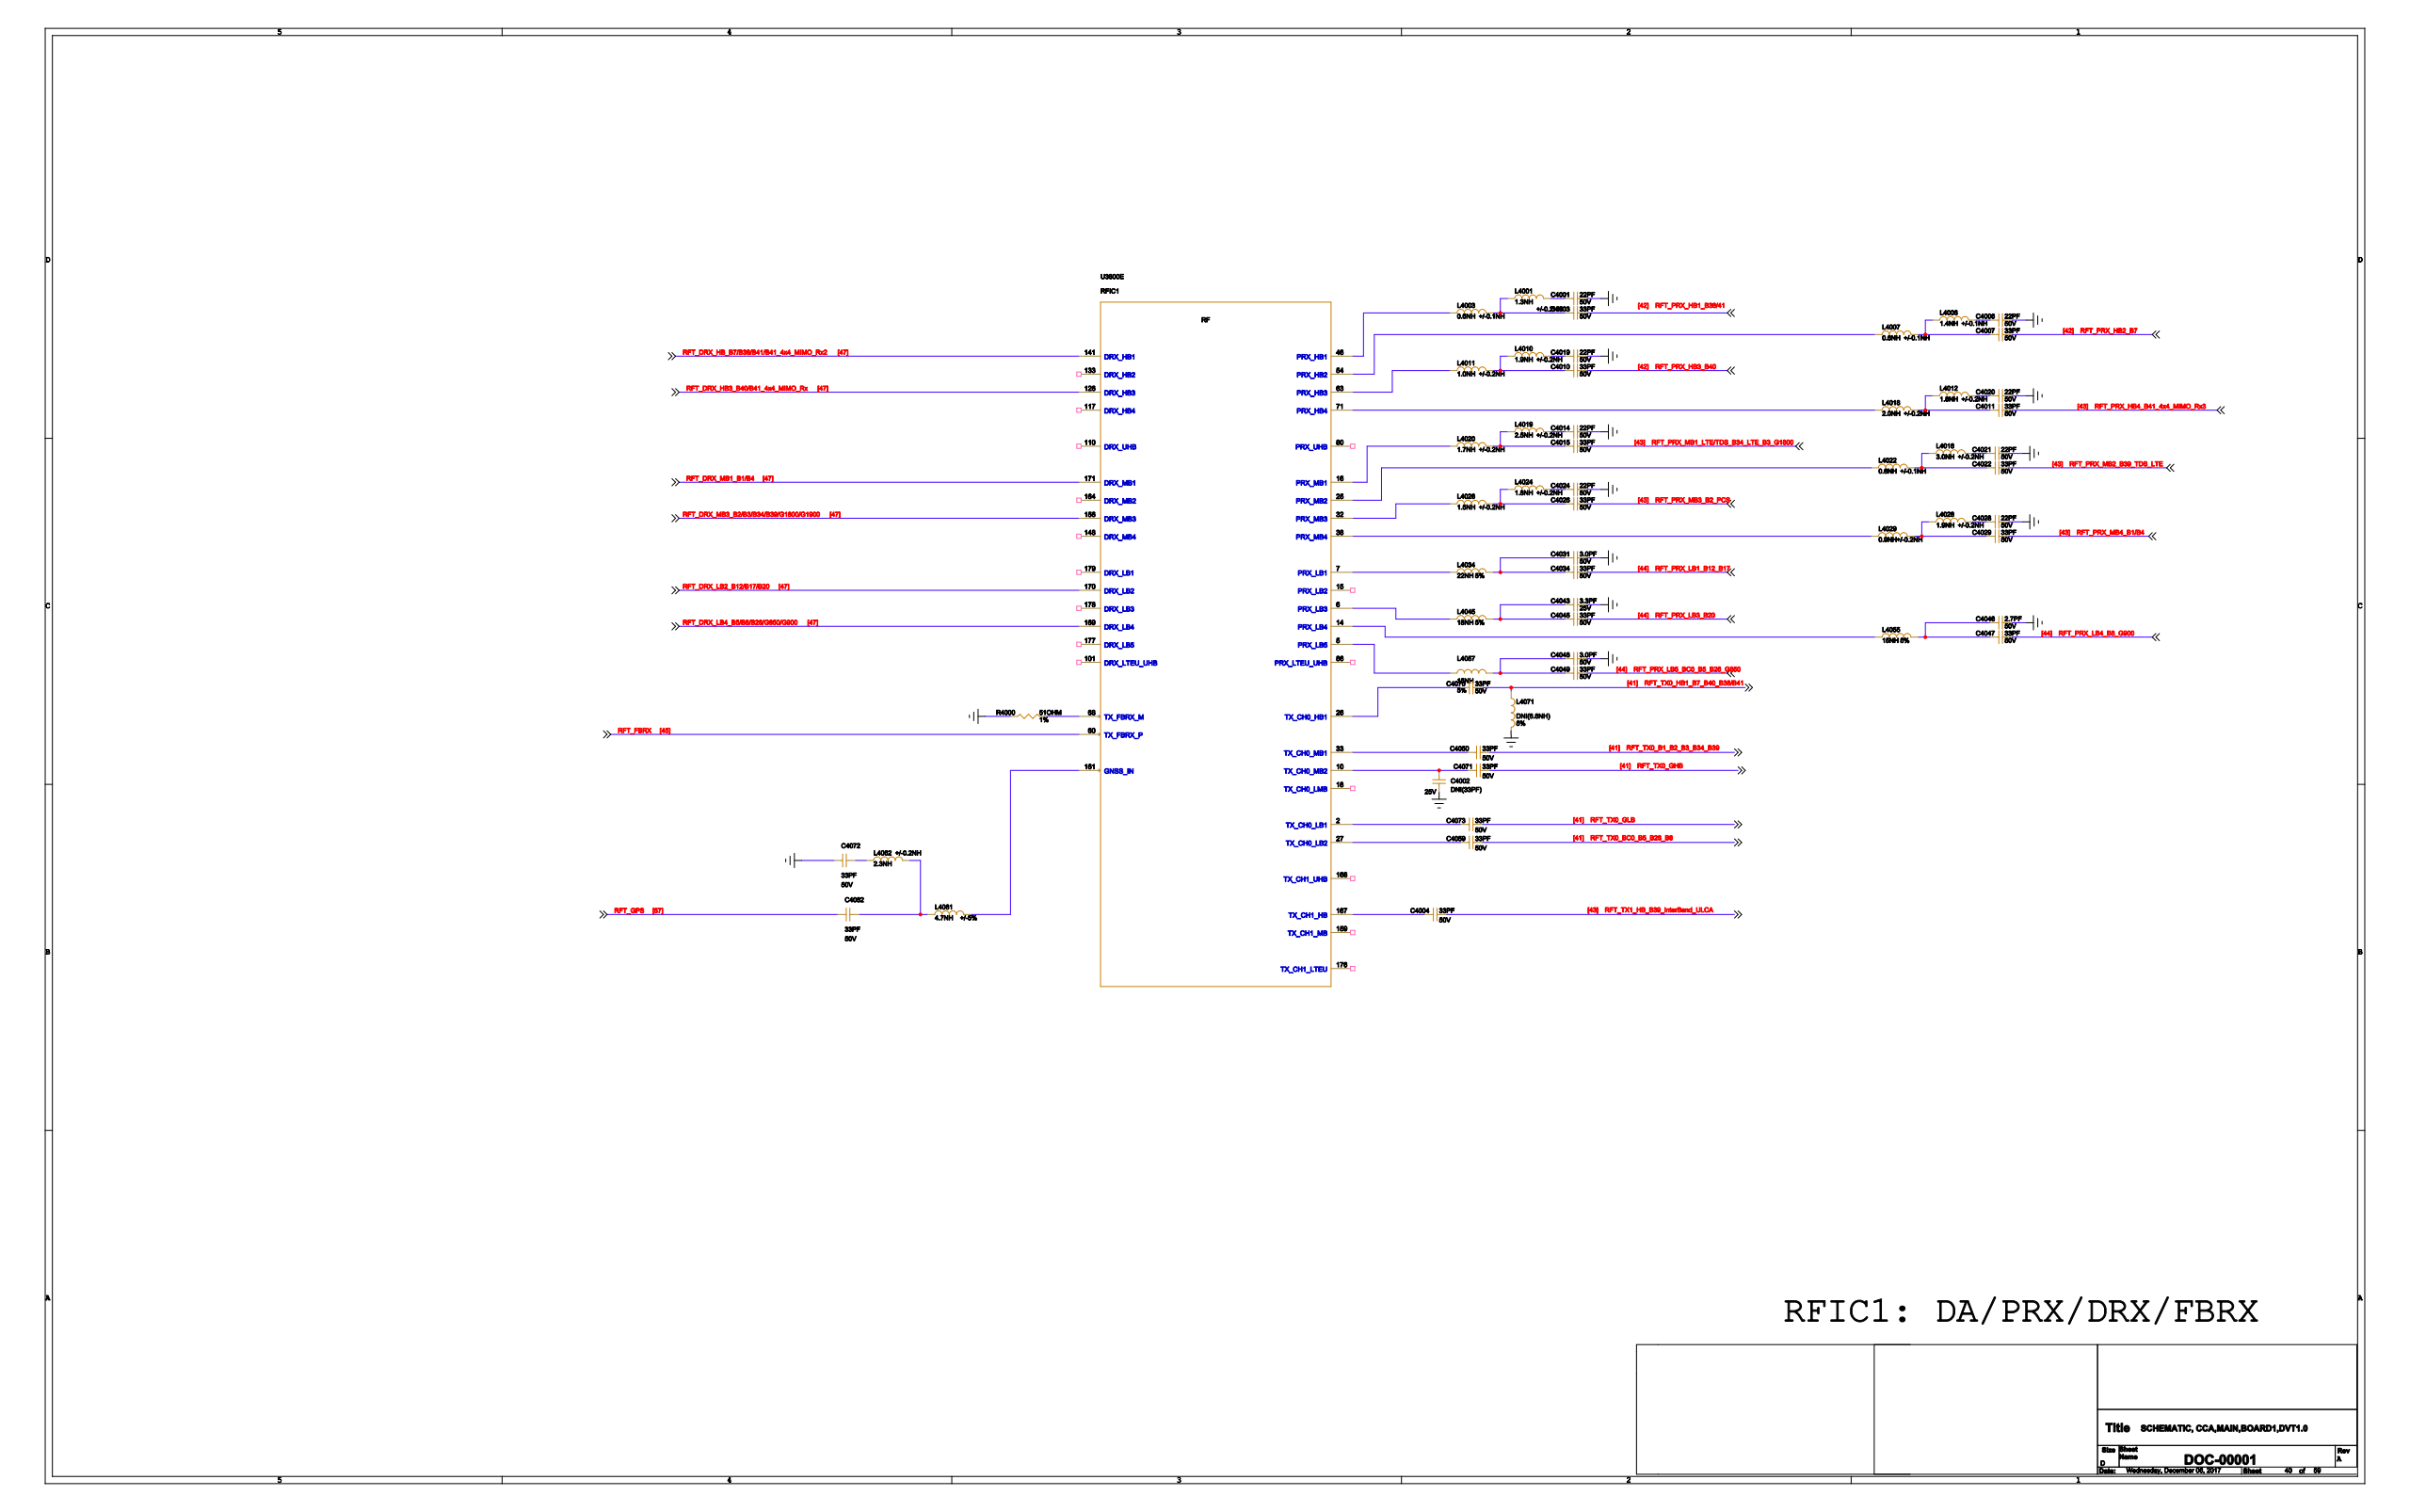Circuit board | KiCad | 1657 parts | 1365 nets | one sheet of the schematic
Parts on this sheet (reference | value | footprint):
C4001
C4002
C4003
C4004
C4006
C4007
C4010
C4011
C4014
C4015
C4019
C4020
C4021
C4022
C4024
C4026
C4028
C4029
C4031
C4034
C4043
C4045
C4046
C4047
C4048
C4049
C4050
C4059
C4062
C4070
C4071
C4072
C4073
L4001
L4003
L4006
L4007
L4010
L4011
L4012
L4016
L4018
L4019
L4020
L4022
L4024
L4026
L4028
L4029
L4034
L4045
L4055
L4057
L4061
L4062
L4071
R4000
U3800
Nets of these parts (net: part-pin ...):
GND: C4001-2 C4002-1 C4006-2 C4014-2 C4019-2 C4020-2 C4021-2 C4024-2 C4028-2 C4031-2 C4043-2 C4046-2 C4048-2 C4072-1 L4071-2 R4000-1 U3800-1 U3800-4 U3800-40
N42474209: C4031-1 C4034-1 L4034-2
RX_LB1_B12_B17: C4034-2
N42473365: C4073-1 U3800-2
RFT_TX0_GLB: C4073-2
N42473857: L4022-1 U3800-25
N42474033: C4022-1 L4016-1 L4022-2
N42474137: C4024-1 L4024-2
N42473873: L4029-1 U3800-38
N42474149: C4029-1 L4028-1 L4029-2
N42474119: C4026-1 L4024-1 L4026-2
N42473849: C4019-1 L4010-2
N42473276: C4002-2 C4071-1 U3800-10
RFT_TX0_GHB: C4071-2
N42473340: C4070-1 U3800-26
B7_B40_B38/B41: C4070-2 L4071-1
N42473847: C4010-1 L4010-1 L4011-2
FT_PRX_HB3_B40: C4010-2
RX_LB4_B8_G900: C4047-2
N42474251: C4043-1 C4045-1 L4045-2
N42473389: C4050-1 U3800-33
_B2_B3_B34_B39: C4050-2
PRX_MB3_B2_PCS: C4026-2
RFT_FBRX: U3800-60
RFT_PRX_HB2_B7: C4007-2
N42474181: C4028-1 L4028-2
B2_B39_TDS_LTE: C4022-2
N42473737: C4007-1 L4006-1 L4007-2
N42473745: C4006-1 L4006-2
_PRX_MB4_B1/B4: C4029-2
_BC0_B5_B26_B8: C4059-2
INTERBAND_ULCA: C4004-2
N42473785: C4001-1 L4001-2
RFT_GPS: C4062-1
N42473188: C4062-2 L4061-2 L4062-2
N42473783: C4003-1 L4001-1 L4003-2
PRX_HB1_B38/41: C4003-2
N42473971: C4015-1 L4019-1 L4020-2
N42473989: C4014-1 L4019-2
FT_PRX_LB3_B20: C4045-2
N42474379: C4048-1 C4049-1 L4057-2
C0_B5_B26_G850: C4049-2
1_4X4_MIMO_RX3: C4011-2
N42473457: L4045-1 U3800-6
N23267517: C4072-2 L4062-1
N42473356: C4059-1 U3800-27
N42473885: L4003-1 U3800-46
N42474335: C4046-1 C4047-1 L4055-2
N42473461: L4057-1 U3800-5
N42473871: L4034-1 U3800-7
N42473881: L4055-1 U3800-14
N42473859: L4020-1 U3800-16
N42473863: L4026-1 U3800-32
N42473875: L4007-1 U3800-54
N42473391: L4011-1 U3800-63
N42475013: R4000-2 U3800-68
N42473160: L4018-1 U3800-71
N42473220: L4061-1 U3800-161
N43198548: C4004-1 U3800-167
N42473945: C4020-1 L4012-2
N42473927: C4011-1 L4012-1 L4018-2
DS_B34_LTE_B3_: C4015-2
N42474053: C4021-1 L4016-2